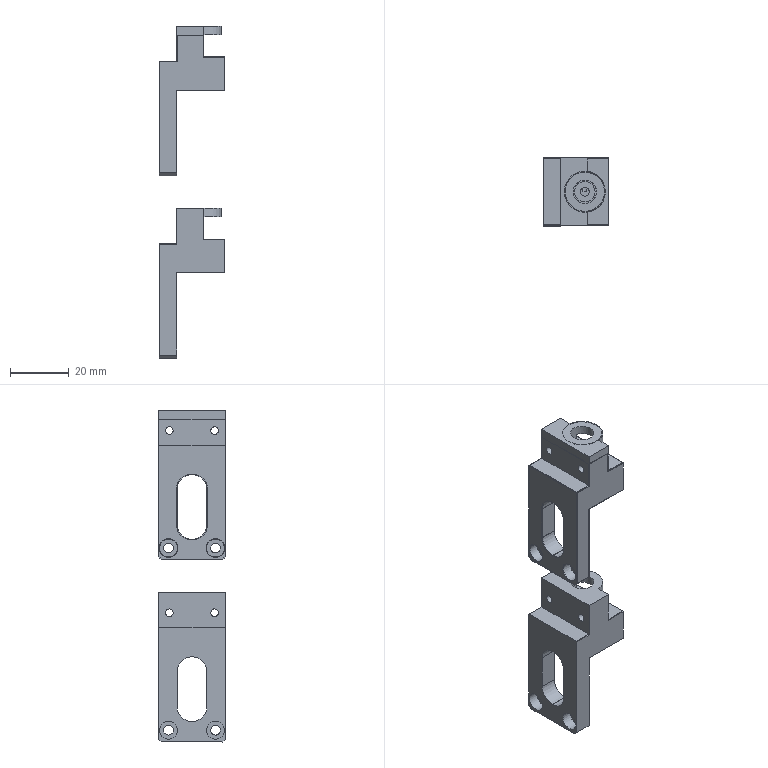Part | 3 solids | 211 faces | box 22.4 x 23 x 113 mm | volume 29189 mm3 | plane 144 | cylinder 48 | cone 19 | commonest cylinder face diameters 10 x12 2.6 x6 3 x6 3.3 x6 6.1 x6 4.2 x3